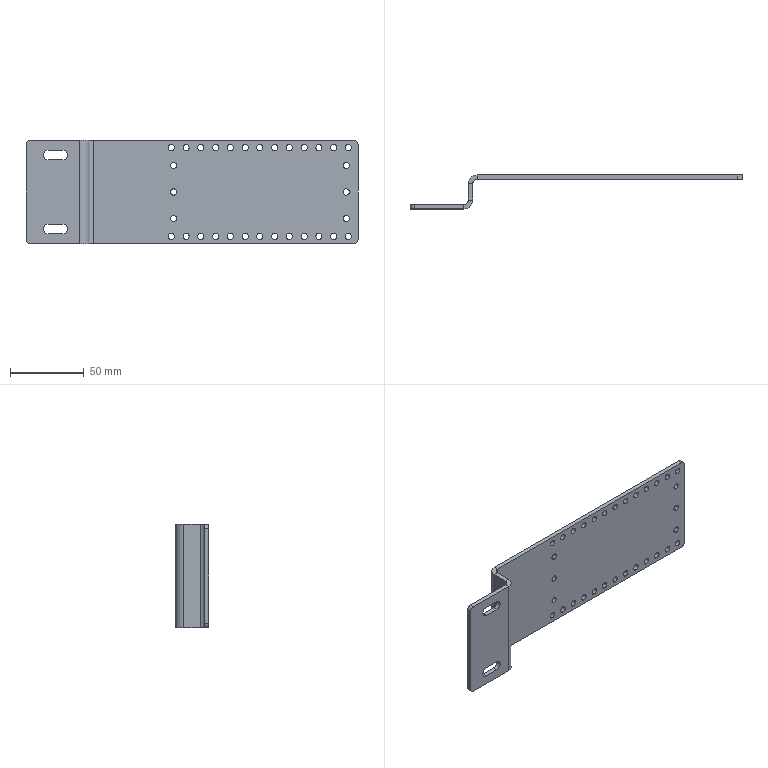Part | SolidWorks | features HoleWzd 3, Fillet 1, FlatPattern 1, ICE 1, Jog 1, SMBaseFlange 1, SheetMetal 1 | 1 solid | 98 faces | box 225 x 23 x 70 mm | volume 48684 mm3 | cylinder 76 | plane 22 | commonest cylinder face diameters 4.2 x64 6 x6 6.6 x4 12 x2